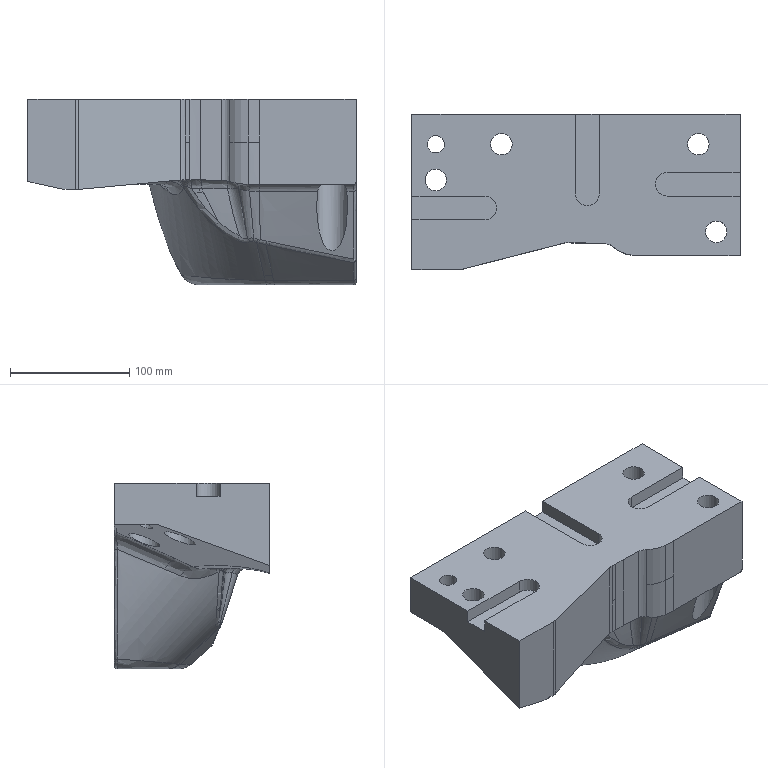Part | STEP file | lll_id70_x_t | 1 solid | 106 faces | box 275 x 130 x 155.537 mm | volume 2917395 mm3 | spline 53 | plane 25 | cylinder 22 | other 4 | cone 1 | torus 1 | commonest cylinder face diameters 20 x6 4 x4 18.009 x4 26.007 x4 14.505 x2 21 x1